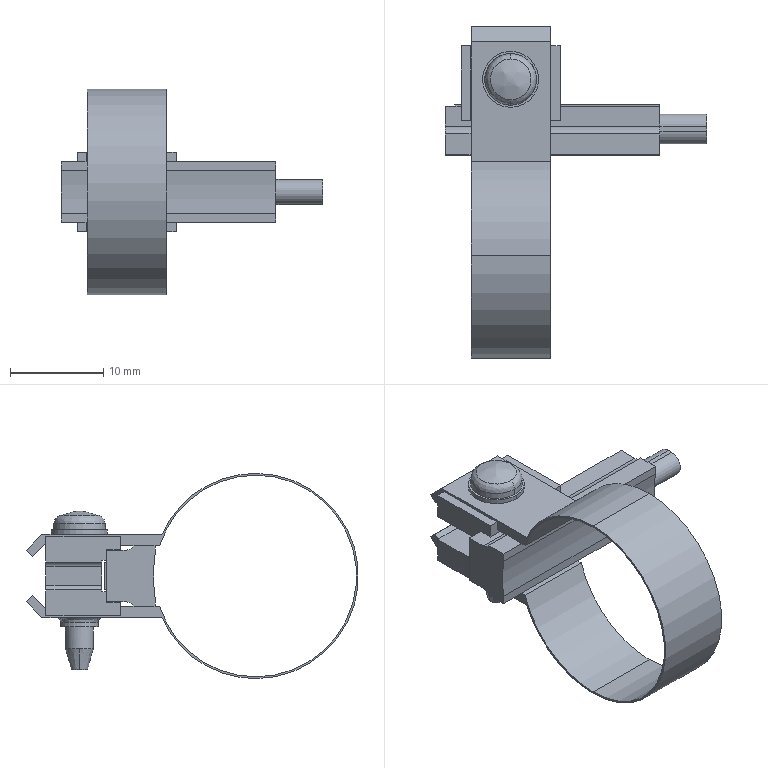Part | STEP file | _CM2-Z_D-M9NW_BM5-020(20_75) | 1 solid | 113 faces | box 28 x 35.624 x 22 mm | volume 1588 mm3 | plane 76 | cylinder 28 | spline 5 | cone 4 | commonest cylinder face diameters 2 x5 1 x4 4 x4 21.6 x3 22 x3 2.5 x2